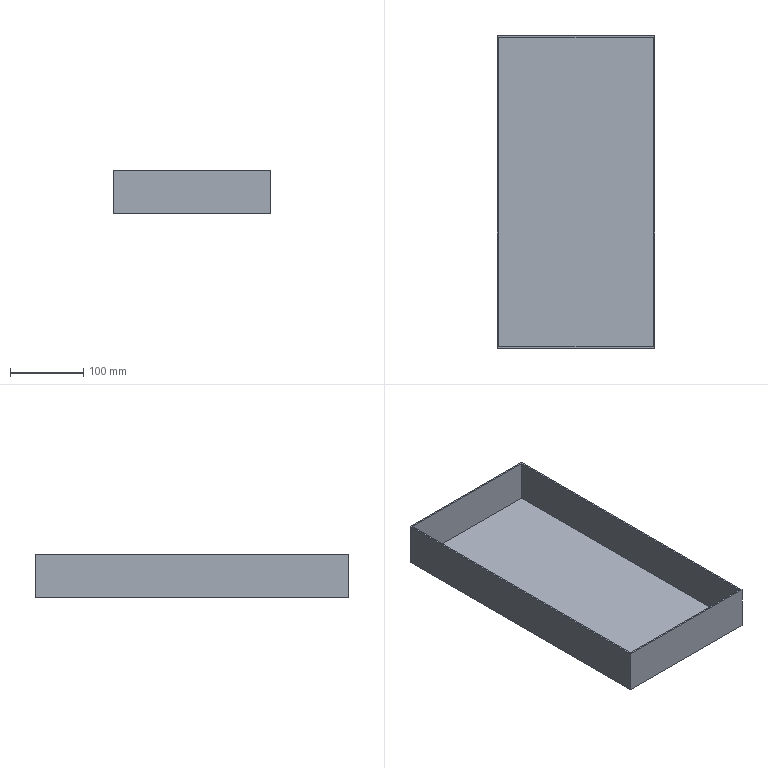Part | NX | features solid 2 | 1 solid | 11 faces | box 215 x 427.059 x 60 mm | volume 331665 mm3 | plane 9 | spline 2
STEP:
#1=CARTESIAN_POINT('',(-250.,-125.,-255.));
#2=VERTEX_POINT('',#1);
#3=CARTESIAN_POINT('',(-35.,-125.,-255.));
#4=VERTEX_POINT('',#3);
#5=CARTESIAN_POINT('',(-530.,-125.,-255.));
#6=DIRECTION('',(-1.,0.,0.));
#7=VECTOR('',#6,1000.);
#8=LINE('',#5,#7);
#9=EDGE_CURVE('',#2,#4,#8,.F.);
#10=ORIENTED_EDGE('',*,*,#9,.T.);
#11=CARTESIAN_POINT('',(-35.,302.059,-255.));
#12=VERTEX_POINT('',#11);
#13=CARTESIAN_POINT('',(-35.,-440.,-255.));
#14=DIRECTION('',(0.,1.,0.));
#15=VECTOR('',#14,1000.);
#16=LINE('',#13,#15);
#17=EDGE_CURVE('',#12,#4,#16,.F.);
#18=ORIENTED_EDGE('',*,*,#17,.F.);
#19=CARTESIAN_POINT('',(-250.,302.059,-255.));
#20=VERTEX_POINT('',#19);
#21=CARTESIAN_POINT('',(-250.,302.059,-255.));
#22=CARTESIAN_POINT('',(-178.333,302.059,-255.));
#23=CARTESIAN_POINT('',(-106.667,302.059,-255.));
#24=CARTESIAN_POINT('',(-35.,302.059,-255.));
#25=B_SPLINE_CURVE_WITH_KNOTS('',3,(#21,#22,#23,#24),.UNSPECIFIED.,.F.,.F.,(4,4),(0.,0.215),.UNSPECIFIED.);
#26=EDGE_CURVE('',#20,#12,#25,.T.);
#27=ORIENTED_EDGE('',*,*,#26,.F.);
#28=CARTESIAN_POINT('',(-250.,-440.,-255.));
#29=DIRECTION('',(0.,1.,0.));
#30=VECTOR('',#29,1000.);
#31=LINE('',#28,#30);
#32=EDGE_CURVE('',#20,#2,#31,.F.);
#33=ORIENTED_EDGE('',*,*,#32,.T.);
#34=EDGE_LOOP('',(#10,#18,#27,#33));
#35=FACE_BOUND('',#34,.T.);
#36=CARTESIAN_POINT('',(-248.,-123.,-255.));
#37=VERTEX_POINT('',#36);
#38=CARTESIAN_POINT('',(-37.,-123.,-255.));
#39=VERTEX_POINT('',#38);
#40=CARTESIAN_POINT('',(-530.,-123.,-255.));
#41=DIRECTION('',(-1.,0.,0.));
#42=VECTOR('',#41,1000.);
#43=LINE('',#40,#42);
#44=EDGE_CURVE('',#37,#39,#43,.F.);
#45=ORIENTED_EDGE('',*,*,#44,.F.);
#46=CARTESIAN_POINT('',(-248.,300.059,-255.));
#47=VERTEX_POINT('',#46);
#48=CARTESIAN_POINT('',(-248.,-440.,-255.));
#49=DIRECTION('',(0.,1.,0.));
#50=VECTOR('',#49,1000.);
#51=LINE('',#48,#50);
#52=EDGE_CURVE('',#47,#37,#51,.F.);
#53=ORIENTED_EDGE('',*,*,#52,.F.);
#54=CARTESIAN_POINT('',(-37.,300.059,-255.));
#55=VERTEX_POINT('',#54);
#56=CARTESIAN_POINT('',(-248.,300.059,-255.));
#57=CARTESIAN_POINT('',(-177.667,300.059,-255.));
#58=CARTESIAN_POINT('',(-107.333,300.059,-255.));
#59=CARTESIAN_POINT('',(-37.,300.059,-255.));
#60=B_SPLINE_CURVE_WITH_KNOTS('',3,(#56,#57,#58,#59),.UNSPECIFIED.,.F.,.F.,(4,4),(0.,0.211),.UNSPECIFIED.);
#61=EDGE_CURVE('',#47,#55,#60,.T.);
#62=ORIENTED_EDGE('',*,*,#61,.T.);
#63=CARTESIAN_POINT('',(-37.,-440.,-255.));
#64=DIRECTION('',(0.,1.,0.));
#65=VECTOR('',#64,1000.);
#66=LINE('',#63,#65);
#67=EDGE_CURVE('',#55,#39,#66,.F.);
#68=ORIENTED_EDGE('',*,*,#67,.T.);
#69=EDGE_LOOP('',(#45,#53,#62,#68));
#70=FACE_BOUND('',#69,.T.);
#71=CARTESIAN_POINT('',(-1030.,-440.,-255.));
#72=DIRECTION('',(0.,0.,1.));
#73=DIRECTION('',(0.,1.,0.));
#74=AXIS2_PLACEMENT_3D('',#71,#72,#73);
#75=PLANE('',#74);
#76=ADVANCED_FACE('',(#35,#70),#75,.T.);
#77=ORIENTED_EDGE('',*,*,#9,.F.);
#78=CARTESIAN_POINT('',(-250.,-125.,-315.));
#79=VERTEX_POINT('',#78);
#80=CARTESIAN_POINT('',(-250.,-125.,-315.));
#81=DIRECTION('',(0.,0.,1.));
#82=VECTOR('',#81,1000.);
#83=LINE('',#80,#82);
#84=EDGE_CURVE('',#79,#2,#83,.T.);
#85=ORIENTED_EDGE('',*,*,#84,.F.);
#86=CARTESIAN_POINT('',(-35.,-125.,-315.));
#87=VERTEX_POINT('',#86);
#88=CARTESIAN_POINT('',(-530.,-125.,-315.));
#89=DIRECTION('',(-1.,0.,0.));
#90=VECTOR('',#89,1000.);
#91=LINE('',#88,#90);
#92=EDGE_CURVE('',#79,#87,#91,.F.);
#93=ORIENTED_EDGE('',*,*,#92,.T.);
#94=CARTESIAN_POINT('',(-35.,-125.,-315.));
#95=DIRECTION('',(0.,0.,1.));
#96=VECTOR('',#95,1000.);
#97=LINE('',#94,#96);
#98=EDGE_CURVE('',#87,#4,#97,.T.);
#99=ORIENTED_EDGE('',*,*,#98,.T.);
#100=EDGE_LOOP('',(#77,#85,#93,#99));
#101=FACE_BOUND('',#100,.T.);
#102=CARTESIAN_POINT('',(-530.,-125.,-315.));
#103=DIRECTION('',(0.,-1.,0.));
#104=DIRECTION('',(0.,0.,-1.));
#105=AXIS2_PLACEMENT_3D('',#102,#103,#104);
#106=PLANE('',#105);
#107=ADVANCED_FACE('',(#101),#106,.T.);
#108=ORIENTED_EDGE('',*,*,#32,.F.);
#109=CARTESIAN_POINT('',(-250.,302.059,-315.));
#110=VERTEX_POINT('',#109);
#111=CARTESIAN_POINT('',(-250.,302.059,-285.));
#112=DIRECTION('',(0.,0.,1.));
#113=VECTOR('',#112,1000.);
#114=LINE('',#111,#113);
#115=EDGE_CURVE('',#110,#20,#114,.T.);
#116=ORIENTED_EDGE('',*,*,#115,.F.);
#117=CARTESIAN_POINT('',(-250.,-440.,-315.));
#118=DIRECTION('',(0.,1.,0.));
#119=VECTOR('',#118,1000.);
#120=LINE('',#117,#119);
#121=EDGE_CURVE('',#110,#79,#120,.F.);
#122=ORIENTED_EDGE('',*,*,#121,.T.);
#123=ORIENTED_EDGE('',*,*,#84,.T.);
#124=EDGE_LOOP('',(#108,#116,#122,#123));
#125=FACE_BOUND('',#124,.T.);
#126=CARTESIAN_POINT('',(-250.,-440.,-315.));
#127=DIRECTION('',(-1.,0.,0.));
#128=DIRECTION('',(0.,0.,1.));
#129=AXIS2_PLACEMENT_3D('',#126,#127,#128);
#130=PLANE('',#129);
#131=ADVANCED_FACE('',(#125),#130,.T.);
#132=ORIENTED_EDGE('',*,*,#26,.T.);
#133=CARTESIAN_POINT('',(-35.,302.059,-315.));
#134=VERTEX_POINT('',#133);
#135=CARTESIAN_POINT('',(-35.,302.059,-285.));
#136=DIRECTION('',(0.,0.,1.));
#137=VECTOR('',#136,1000.);
#138=LINE('',#135,#137);
#139=EDGE_CURVE('',#134,#12,#138,.T.);
#140=ORIENTED_EDGE('',*,*,#139,.F.);
#141=CARTESIAN_POINT('',(-250.,302.059,-315.));
#142=CARTESIAN_POINT('',(-178.333,302.059,-315.));
#143=CARTESIAN_POINT('',(-106.667,302.059,-315.));
#144=CARTESIAN_POINT('',(-35.,302.059,-315.));
#145=B_SPLINE_CURVE_WITH_KNOTS('',3,(#141,#142,#143,#144),.UNSPECIFIED.,.F.,.F.,(4,4),(0.,0.215),.UNSPECIFIED.);
#146=EDGE_CURVE('',#110,#134,#145,.T.);
#147=ORIENTED_EDGE('',*,*,#146,.F.);
#148=ORIENTED_EDGE('',*,*,#115,.T.);
#149=EDGE_LOOP('',(#132,#140,#147,#148));
#150=FACE_BOUND('',#149,.T.);
#151=CARTESIAN_POINT('',(-35.,302.059,-315.));
#152=CARTESIAN_POINT('',(-35.,302.059,-255.));
#153=CARTESIAN_POINT('',(-106.667,302.059,-315.));
#154=CARTESIAN_POINT('',(-106.667,302.059,-255.));
#155=CARTESIAN_POINT('',(-178.333,302.059,-315.));
#156=CARTESIAN_POINT('',(-178.333,302.059,-255.));
#157=CARTESIAN_POINT('',(-250.,302.059,-315.));
#158=CARTESIAN_POINT('',(-250.,302.059,-255.));
#159=B_SPLINE_SURFACE_WITH_KNOTS('',3,1,((#151,#152),(#153,#154),(#155,#156),(#157,#158)),.SURF_OF_LINEAR_EXTRUSION.,.F.,.F.,.F.,(4,4),(2,2),(0.03139,0.2242),(0.,1.),.PIECEWISE_BEZIER_KNOTS.);
#160=ADVANCED_FACE('',(#150),#159,.T.);
#161=ORIENTED_EDGE('',*,*,#17,.T.);
#162=ORIENTED_EDGE('',*,*,#98,.F.);
#163=CARTESIAN_POINT('',(-35.,-440.,-315.));
#164=DIRECTION('',(0.,1.,0.));
#165=VECTOR('',#164,1000.);
#166=LINE('',#163,#165);
#167=EDGE_CURVE('',#134,#87,#166,.F.);
#168=ORIENTED_EDGE('',*,*,#167,.F.);
#169=ORIENTED_EDGE('',*,*,#139,.T.);
#170=EDGE_LOOP('',(#161,#162,#168,#169));
#171=FACE_BOUND('',#170,.T.);
#172=CARTESIAN_POINT('',(-35.,-440.,-315.));
#173=DIRECTION('',(-1.,0.,0.));
#174=DIRECTION('',(0.,0.,1.));
#175=AXIS2_PLACEMENT_3D('',#172,#173,#174);
#176=PLANE('',#175);
#177=ADVANCED_FACE('',(#171),#176,.F.);
#178=ORIENTED_EDGE('',*,*,#92,.F.);
#179=ORIENTED_EDGE('',*,*,#121,.F.);
#180=ORIENTED_EDGE('',*,*,#146,.T.);
#181=ORIENTED_EDGE('',*,*,#167,.T.);
#182=EDGE_LOOP('',(#178,#179,#180,#181));
#183=FACE_BOUND('',#182,.T.);
#184=CARTESIAN_POINT('',(-1030.,-440.,-315.));
#185=DIRECTION('',(0.,0.,1.));
#186=DIRECTION('',(0.,1.,0.));
#187=AXIS2_PLACEMENT_3D('',#184,#185,#186);
#188=PLANE('',#187);
#189=ADVANCED_FACE('',(#183),#188,.F.);
#190=ORIENTED_EDGE('',*,*,#44,.T.);
#191=CARTESIAN_POINT('',(-37.,-123.,-313.));
#192=VERTEX_POINT('',#191);
#193=CARTESIAN_POINT('',(-37.,-123.,-315.));
#194=DIRECTION('',(0.,0.,1.));
#195=VECTOR('',#194,1000.);
#196=LINE('',#193,#195);
#197=EDGE_CURVE('',#192,#39,#196,.T.);
#198=ORIENTED_EDGE('',*,*,#197,.F.);
#199=CARTESIAN_POINT('',(-248.,-123.,-313.));
#200=VERTEX_POINT('',#199);
#201=CARTESIAN_POINT('',(-530.,-123.,-313.));
#202=DIRECTION('',(-1.,0.,0.));
#203=VECTOR('',#202,1000.);
#204=LINE('',#201,#203);
#205=EDGE_CURVE('',#200,#192,#204,.F.);
#206=ORIENTED_EDGE('',*,*,#205,.F.);
#207=CARTESIAN_POINT('',(-248.,-123.,-315.));
#208=DIRECTION('',(0.,0.,1.));
#209=VECTOR('',#208,1000.);
#210=LINE('',#207,#209);
#211=EDGE_CURVE('',#200,#37,#210,.T.);
#212=ORIENTED_EDGE('',*,*,#211,.T.);
#213=EDGE_LOOP('',(#190,#198,#206,#212));
#214=FACE_BOUND('',#213,.T.);
#215=CARTESIAN_POINT('',(-530.,-123.,-315.));
#216=DIRECTION('',(0.,-1.,0.));
#217=DIRECTION('',(0.,0.,-1.));
#218=AXIS2_PLACEMENT_3D('',#215,#216,#217);
#219=PLANE('',#218);
#220=ADVANCED_FACE('',(#214),#219,.F.);
#221=ORIENTED_EDGE('',*,*,#52,.T.);
#222=ORIENTED_EDGE('',*,*,#211,.F.);
#223=CARTESIAN_POINT('',(-248.,300.059,-313.));
#224=VERTEX_POINT('',#223);
#225=CARTESIAN_POINT('',(-248.,-440.,-313.));
#226=DIRECTION('',(0.,1.,0.));
#227=VECTOR('',#226,1000.);
#228=LINE('',#225,#227);
#229=EDGE_CURVE('',#224,#200,#228,.F.);
#230=ORIENTED_EDGE('',*,*,#229,.F.);
#231=CARTESIAN_POINT('',(-248.,300.059,-313.));
#232=DIRECTION('',(0.,0.,1.));
#233=VECTOR('',#232,1000.);
#234=LINE('',#231,#233);
#235=EDGE_CURVE('',#224,#47,#234,.T.);
#236=ORIENTED_EDGE('',*,*,#235,.T.);
#237=EDGE_LOOP('',(#221,#222,#230,#236));
#238=FACE_BOUND('',#237,.T.);
#239=CARTESIAN_POINT('',(-248.,-440.,-315.));
#240=DIRECTION('',(-1.,0.,0.));
#241=DIRECTION('',(0.,0.,1.));
#242=AXIS2_PLACEMENT_3D('',#239,#240,#241);
#243=PLANE('',#242);
#244=ADVANCED_FACE('',(#238),#243,.F.);
#245=ORIENTED_EDGE('',*,*,#61,.F.);
#246=ORIENTED_EDGE('',*,*,#235,.F.);
#247=CARTESIAN_POINT('',(-37.,300.059,-313.));
#248=VERTEX_POINT('',#247);
#249=CARTESIAN_POINT('',(-248.,300.059,-313.));
#250=CARTESIAN_POINT('',(-177.667,300.059,-313.));
#251=CARTESIAN_POINT('',(-107.333,300.059,-313.));
#252=CARTESIAN_POINT('',(-37.,300.059,-313.));
#253=B_SPLINE_CURVE_WITH_KNOTS('',3,(#249,#250,#251,#252),.UNSPECIFIED.,.F.,.F.,(4,4),(0.,0.211),.UNSPECIFIED.);
#254=EDGE_CURVE('',#224,#248,#253,.T.);
#255=ORIENTED_EDGE('',*,*,#254,.T.);
#256=CARTESIAN_POINT('',(-37.,300.059,-313.));
#257=DIRECTION('',(0.,0.,1.));
#258=VECTOR('',#257,1000.);
#259=LINE('',#256,#258);
#260=EDGE_CURVE('',#248,#55,#259,.T.);
#261=ORIENTED_EDGE('',*,*,#260,.T.);
#262=EDGE_LOOP('',(#245,#246,#255,#261));
#263=FACE_BOUND('',#262,.T.);
#264=CARTESIAN_POINT('',(-37.,300.059,-313.));
#265=CARTESIAN_POINT('',(-37.,300.059,-255.));
#266=CARTESIAN_POINT('',(-107.333,300.059,-313.));
#267=CARTESIAN_POINT('',(-107.333,300.059,-255.));
#268=CARTESIAN_POINT('',(-177.667,300.059,-313.));
#269=CARTESIAN_POINT('',(-177.667,300.059,-255.));
#270=CARTESIAN_POINT('',(-248.,300.059,-313.));
#271=CARTESIAN_POINT('',(-248.,300.059,-255.));
#272=B_SPLINE_SURFACE_WITH_KNOTS('',3,1,((#264,#265),(#266,#267),(#268,#269),(#270,#271)),.SURF_OF_LINEAR_EXTRUSION.,.F.,.F.,.F.,(4,4),(2,2),(0.,1.),(0.,1.),.PIECEWISE_BEZIER_KNOTS.);
#273=ADVANCED_FACE('',(#263),#272,.F.);
#274=ORIENTED_EDGE('',*,*,#67,.F.);
#275=ORIENTED_EDGE('',*,*,#260,.F.);
#276=CARTESIAN_POINT('',(-37.,-440.,-313.));
#277=DIRECTION('',(0.,1.,0.));
#278=VECTOR('',#277,1000.);
#279=LINE('',#276,#278);
#280=EDGE_CURVE('',#248,#192,#279,.F.);
#281=ORIENTED_EDGE('',*,*,#280,.T.);
#282=ORIENTED_EDGE('',*,*,#197,.T.);
#283=EDGE_LOOP('',(#274,#275,#281,#282));
#284=FACE_BOUND('',#283,.T.);
#285=CARTESIAN_POINT('',(-37.,-440.,-315.));
#286=DIRECTION('',(-1.,0.,0.));
#287=DIRECTION('',(0.,0.,1.));
#288=AXIS2_PLACEMENT_3D('',#285,#286,#287);
#289=PLANE('',#288);
#290=ADVANCED_FACE('',(#284),#289,.T.);
#291=ORIENTED_EDGE('',*,*,#205,.T.);
#292=ORIENTED_EDGE('',*,*,#280,.F.);
#293=ORIENTED_EDGE('',*,*,#254,.F.);
#294=ORIENTED_EDGE('',*,*,#229,.T.);
#295=EDGE_LOOP('',(#291,#292,#293,#294));
#296=FACE_BOUND('',#295,.T.);
#297=CARTESIAN_POINT('',(-1030.,-440.,-313.));
#298=DIRECTION('',(0.,0.,1.));
#299=DIRECTION('',(0.,1.,0.));
#300=AXIS2_PLACEMENT_3D('',#297,#298,#299);
#301=PLANE('',#300);
#302=ADVANCED_FACE('',(#296),#301,.T.);
#303=CLOSED_SHELL('',(#76,#107,#131,#160,#177,#189,#220,#244,#273,#290,#302));
#304=MANIFOLD_SOLID_BREP('',#303);
#305=(LENGTH_UNIT()NAMED_UNIT(*)SI_UNIT(.MILLI.,.METRE.));
#306=UNCERTAINTY_MEASURE_WITH_UNIT(LENGTH_MEASURE(0.0508),#305,'','');
#307=(NAMED_UNIT(*)PLANE_ANGLE_UNIT()SI_UNIT($,.RADIAN.));
#308=(NAMED_UNIT(*)SI_UNIT($,.STERADIAN.)SOLID_ANGLE_UNIT());
#309=(GEOMETRIC_REPRESENTATION_CONTEXT(3)GLOBAL_UNCERTAINTY_ASSIGNED_CONTEXT((#306))GLOBAL_UNIT_ASSIGNED_CONTEXT((#305,#307,#308))REPRESENTATION_CONTEXT('',''));
#310=ADVANCED_BREP_SHAPE_REPRESENTATION('',(#304),#309);